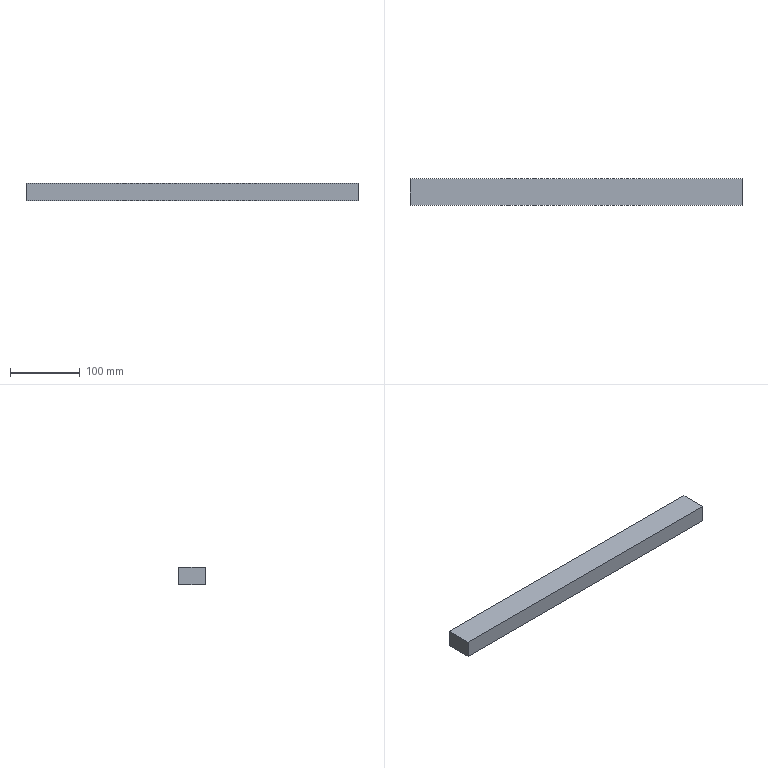Part | SolidWorks | features Extrusion 1 | 1 solid | 6 faces | box 475 x 38 x 25 mm | volume 451250 mm3 | plane 6
STEP:
#1=CARTESIAN_POINT('',(237.5,-19.,0.));
#2=VERTEX_POINT('',#1);
#3=CARTESIAN_POINT('',(237.5,19.,0.));
#4=VERTEX_POINT('',#3);
#5=CARTESIAN_POINT('',(237.5,19.,0.));
#6=DIRECTION('',(0.,1.,0.));
#7=VECTOR('',#6,1000.);
#8=LINE('',#5,#7);
#9=EDGE_CURVE('',#2,#4,#8,.T.);
#10=ORIENTED_EDGE('',*,*,#9,.T.);
#11=CARTESIAN_POINT('',(237.5,19.,25.));
#12=VERTEX_POINT('',#11);
#13=CARTESIAN_POINT('',(237.5,19.,25.));
#14=DIRECTION('',(0.,0.,-1.));
#15=VECTOR('',#14,1000.);
#16=LINE('',#13,#15);
#17=EDGE_CURVE('',#12,#4,#16,.T.);
#18=ORIENTED_EDGE('',*,*,#17,.F.);
#19=CARTESIAN_POINT('',(237.5,-19.,25.));
#20=VERTEX_POINT('',#19);
#21=CARTESIAN_POINT('',(237.5,19.,25.));
#22=DIRECTION('',(0.,1.,0.));
#23=VECTOR('',#22,1000.);
#24=LINE('',#21,#23);
#25=EDGE_CURVE('',#20,#12,#24,.T.);
#26=ORIENTED_EDGE('',*,*,#25,.F.);
#27=CARTESIAN_POINT('',(237.5,-19.,25.));
#28=DIRECTION('',(0.,0.,-1.));
#29=VECTOR('',#28,1000.);
#30=LINE('',#27,#29);
#31=EDGE_CURVE('',#20,#2,#30,.T.);
#32=ORIENTED_EDGE('',*,*,#31,.T.);
#33=EDGE_LOOP('',(#10,#18,#26,#32));
#34=FACE_OUTER_BOUND('',#33,.T.);
#35=CARTESIAN_POINT('',(237.5,19.,25.));
#36=DIRECTION('',(-1.,0.,0.));
#37=DIRECTION('',(0.,0.,1.));
#38=AXIS2_PLACEMENT_3D('',#35,#36,#37);
#39=PLANE('',#38);
#40=ADVANCED_FACE('',(#34),#39,.F.);
#41=CARTESIAN_POINT('',(-237.5,19.,0.));
#42=VERTEX_POINT('',#41);
#43=CARTESIAN_POINT('',(-237.5,19.,0.));
#44=DIRECTION('',(-1.,0.,0.));
#45=VECTOR('',#44,1000.);
#46=LINE('',#43,#45);
#47=EDGE_CURVE('',#4,#42,#46,.T.);
#48=ORIENTED_EDGE('',*,*,#47,.T.);
#49=CARTESIAN_POINT('',(-237.5,19.,25.));
#50=VERTEX_POINT('',#49);
#51=CARTESIAN_POINT('',(-237.5,19.,25.));
#52=DIRECTION('',(0.,0.,-1.));
#53=VECTOR('',#52,1000.);
#54=LINE('',#51,#53);
#55=EDGE_CURVE('',#50,#42,#54,.T.);
#56=ORIENTED_EDGE('',*,*,#55,.F.);
#57=CARTESIAN_POINT('',(-237.5,19.,25.));
#58=DIRECTION('',(-1.,0.,0.));
#59=VECTOR('',#58,1000.);
#60=LINE('',#57,#59);
#61=EDGE_CURVE('',#12,#50,#60,.T.);
#62=ORIENTED_EDGE('',*,*,#61,.F.);
#63=ORIENTED_EDGE('',*,*,#17,.T.);
#64=EDGE_LOOP('',(#48,#56,#62,#63));
#65=FACE_OUTER_BOUND('',#64,.T.);
#66=CARTESIAN_POINT('',(-237.5,19.,25.));
#67=DIRECTION('',(0.,-1.,0.));
#68=DIRECTION('',(0.,0.,-1.));
#69=AXIS2_PLACEMENT_3D('',#66,#67,#68);
#70=PLANE('',#69);
#71=ADVANCED_FACE('',(#65),#70,.F.);
#72=CARTESIAN_POINT('',(-237.5,-19.,0.));
#73=VERTEX_POINT('',#72);
#74=CARTESIAN_POINT('',(-237.5,19.,0.));
#75=DIRECTION('',(0.,-1.,0.));
#76=VECTOR('',#75,1000.);
#77=LINE('',#74,#76);
#78=EDGE_CURVE('',#42,#73,#77,.T.);
#79=ORIENTED_EDGE('',*,*,#78,.T.);
#80=CARTESIAN_POINT('',(-237.5,-19.,25.));
#81=VERTEX_POINT('',#80);
#82=CARTESIAN_POINT('',(-237.5,-19.,25.));
#83=DIRECTION('',(0.,0.,-1.));
#84=VECTOR('',#83,1000.);
#85=LINE('',#82,#84);
#86=EDGE_CURVE('',#81,#73,#85,.T.);
#87=ORIENTED_EDGE('',*,*,#86,.F.);
#88=CARTESIAN_POINT('',(-237.5,19.,25.));
#89=DIRECTION('',(0.,-1.,0.));
#90=VECTOR('',#89,1000.);
#91=LINE('',#88,#90);
#92=EDGE_CURVE('',#50,#81,#91,.T.);
#93=ORIENTED_EDGE('',*,*,#92,.F.);
#94=ORIENTED_EDGE('',*,*,#55,.T.);
#95=EDGE_LOOP('',(#79,#87,#93,#94));
#96=FACE_OUTER_BOUND('',#95,.T.);
#97=CARTESIAN_POINT('',(-237.5,19.,25.));
#98=DIRECTION('',(1.,0.,0.));
#99=DIRECTION('',(0.,0.,-1.));
#100=AXIS2_PLACEMENT_3D('',#97,#98,#99);
#101=PLANE('',#100);
#102=ADVANCED_FACE('',(#96),#101,.F.);
#103=CARTESIAN_POINT('',(-237.5,-19.,0.));
#104=DIRECTION('',(1.,0.,0.));
#105=VECTOR('',#104,1000.);
#106=LINE('',#103,#105);
#107=EDGE_CURVE('',#73,#2,#106,.T.);
#108=ORIENTED_EDGE('',*,*,#107,.T.);
#109=ORIENTED_EDGE('',*,*,#31,.F.);
#110=CARTESIAN_POINT('',(-237.5,-19.,25.));
#111=DIRECTION('',(1.,0.,0.));
#112=VECTOR('',#111,1000.);
#113=LINE('',#110,#112);
#114=EDGE_CURVE('',#81,#20,#113,.T.);
#115=ORIENTED_EDGE('',*,*,#114,.F.);
#116=ORIENTED_EDGE('',*,*,#86,.T.);
#117=EDGE_LOOP('',(#108,#109,#115,#116));
#118=FACE_OUTER_BOUND('',#117,.T.);
#119=CARTESIAN_POINT('',(-237.5,-19.,25.));
#120=DIRECTION('',(0.,1.,0.));
#121=DIRECTION('',(0.,0.,1.));
#122=AXIS2_PLACEMENT_3D('',#119,#120,#121);
#123=PLANE('',#122);
#124=ADVANCED_FACE('',(#118),#123,.F.);
#125=ORIENTED_EDGE('',*,*,#25,.T.);
#126=ORIENTED_EDGE('',*,*,#61,.T.);
#127=ORIENTED_EDGE('',*,*,#92,.T.);
#128=ORIENTED_EDGE('',*,*,#114,.T.);
#129=EDGE_LOOP('',(#125,#126,#127,#128));
#130=FACE_OUTER_BOUND('',#129,.T.);
#131=CARTESIAN_POINT('',(0.,0.,25.));
#132=DIRECTION('',(0.,0.,1.));
#133=DIRECTION('',(1.,0.,0.));
#134=AXIS2_PLACEMENT_3D('',#131,#132,#133);
#135=PLANE('',#134);
#136=ADVANCED_FACE('',(#130),#135,.T.);
#137=ORIENTED_EDGE('',*,*,#9,.F.);
#138=ORIENTED_EDGE('',*,*,#107,.F.);
#139=ORIENTED_EDGE('',*,*,#78,.F.);
#140=ORIENTED_EDGE('',*,*,#47,.F.);
#141=EDGE_LOOP('',(#137,#138,#139,#140));
#142=FACE_OUTER_BOUND('',#141,.T.);
#143=CARTESIAN_POINT('',(0.,0.,0.));
#144=DIRECTION('',(0.,0.,1.));
#145=DIRECTION('',(1.,0.,0.));
#146=AXIS2_PLACEMENT_3D('',#143,#144,#145);
#147=PLANE('',#146);
#148=ADVANCED_FACE('',(#142),#147,.F.);
#149=CLOSED_SHELL('',(#40,#71,#102,#124,#136,#148));
#150=MANIFOLD_SOLID_BREP('',#149);
#151=CARTESIAN_POINT('',(0.,0.,0.));
#152=DIRECTION('',(0.,0.,1.));
#153=DIRECTION('',(1.,0.,0.));
#154=AXIS2_PLACEMENT_3D('',#151,#152,#153);
#155=(LENGTH_UNIT()NAMED_UNIT(*)SI_UNIT(.MILLI.,.METRE.));
#156=UNCERTAINTY_MEASURE_WITH_UNIT(LENGTH_MEASURE(0.00001),#155,'','');
#157=(NAMED_UNIT(*)PLANE_ANGLE_UNIT()SI_UNIT($,.RADIAN.));
#158=(NAMED_UNIT(*)SI_UNIT($,.STERADIAN.)SOLID_ANGLE_UNIT());
#159=(GEOMETRIC_REPRESENTATION_CONTEXT(3)GLOBAL_UNCERTAINTY_ASSIGNED_CONTEXT((#156))GLOBAL_UNIT_ASSIGNED_CONTEXT((#155,#157,#158))REPRESENTATION_CONTEXT('',''));
#160=ADVANCED_BREP_SHAPE_REPRESENTATION('',(#150,#154),#159);